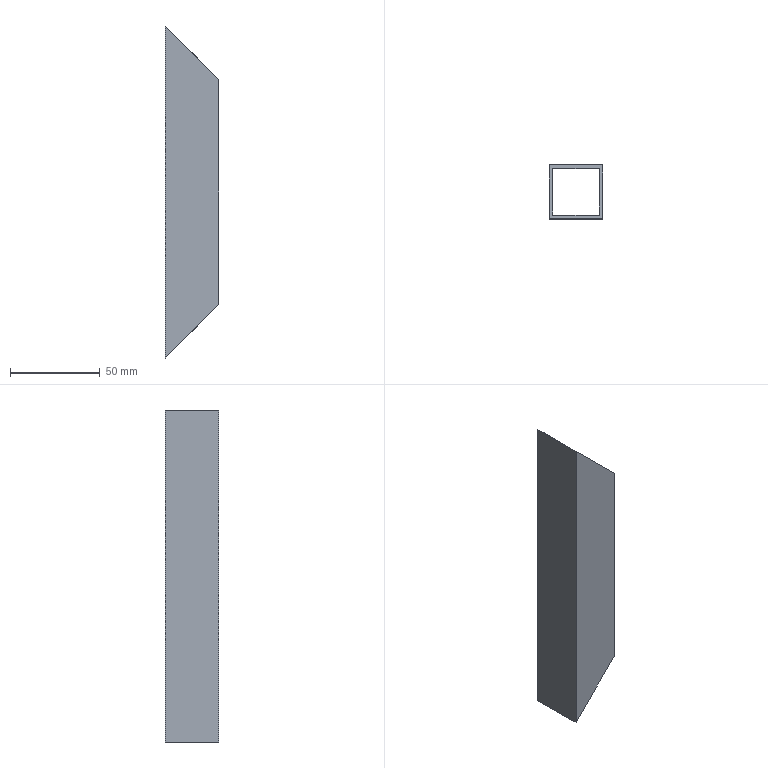Part | SolidWorks | features Extrusion 1, ICE 1 | 1 solid | 10 faces | box 30 x 30 x 185 mm | volume 34720 mm3 | plane 10
STEP:
#1=CARTESIAN_POINT('',(13.,-13.,64.5));
#2=VERTEX_POINT('',#1);
#3=CARTESIAN_POINT('',(-13.,-13.,90.5));
#4=VERTEX_POINT('',#3);
#5=CARTESIAN_POINT('',(-1.,-13.,78.5));
#6=DIRECTION('',(-0.7071,0.,0.7071));
#7=VECTOR('',#6,1000.);
#8=LINE('',#5,#7);
#9=EDGE_CURVE('',#2,#4,#8,.T.);
#10=ORIENTED_EDGE('',*,*,#9,.F.);
#11=CARTESIAN_POINT('',(13.,-13.,-64.5));
#12=VERTEX_POINT('',#11);
#13=CARTESIAN_POINT('',(13.,-13.,92.5));
#14=DIRECTION('',(0.,0.,-1.));
#15=VECTOR('',#14,1000.);
#16=LINE('',#13,#15);
#17=EDGE_CURVE('',#2,#12,#16,.T.);
#18=ORIENTED_EDGE('',*,*,#17,.T.);
#19=CARTESIAN_POINT('',(-13.,-13.,-90.5));
#20=VERTEX_POINT('',#19);
#21=CARTESIAN_POINT('',(91.5,-13.,14.));
#22=DIRECTION('',(0.7071,0.,0.7071));
#23=VECTOR('',#22,1000.);
#24=LINE('',#21,#23);
#25=EDGE_CURVE('',#20,#12,#24,.T.);
#26=ORIENTED_EDGE('',*,*,#25,.F.);
#27=CARTESIAN_POINT('',(-13.,-13.,92.5));
#28=DIRECTION('',(0.,0.,-1.));
#29=VECTOR('',#28,1000.);
#30=LINE('',#27,#29);
#31=EDGE_CURVE('',#4,#20,#30,.T.);
#32=ORIENTED_EDGE('',*,*,#31,.F.);
#33=EDGE_LOOP('',(#10,#18,#26,#32));
#34=FACE_OUTER_BOUND('',#33,.T.);
#35=CARTESIAN_POINT('',(13.,-13.,92.5));
#36=DIRECTION('',(0.,1.,0.));
#37=DIRECTION('',(0.,0.,1.));
#38=AXIS2_PLACEMENT_3D('',#35,#36,#37);
#39=PLANE('',#38);
#40=ADVANCED_FACE('',(#34),#39,.T.);
#41=CARTESIAN_POINT('',(-13.,13.,90.5));
#42=VERTEX_POINT('',#41);
#43=CARTESIAN_POINT('',(-13.,-13.,90.5));
#44=DIRECTION('',(0.,1.,0.));
#45=VECTOR('',#44,1000.);
#46=LINE('',#43,#45);
#47=EDGE_CURVE('',#4,#42,#46,.T.);
#48=ORIENTED_EDGE('',*,*,#47,.F.);
#49=ORIENTED_EDGE('',*,*,#31,.T.);
#50=CARTESIAN_POINT('',(-13.,13.,-90.5));
#51=VERTEX_POINT('',#50);
#52=CARTESIAN_POINT('',(-13.,-13.,-90.5));
#53=DIRECTION('',(0.,-1.,0.));
#54=VECTOR('',#53,1000.);
#55=LINE('',#52,#54);
#56=EDGE_CURVE('',#51,#20,#55,.T.);
#57=ORIENTED_EDGE('',*,*,#56,.F.);
#58=CARTESIAN_POINT('',(-13.,13.,92.5));
#59=DIRECTION('',(0.,0.,-1.));
#60=VECTOR('',#59,1000.);
#61=LINE('',#58,#60);
#62=EDGE_CURVE('',#42,#51,#61,.T.);
#63=ORIENTED_EDGE('',*,*,#62,.F.);
#64=EDGE_LOOP('',(#48,#49,#57,#63));
#65=FACE_OUTER_BOUND('',#64,.T.);
#66=CARTESIAN_POINT('',(-13.,-13.,92.5));
#67=DIRECTION('',(1.,0.,0.));
#68=DIRECTION('',(0.,0.,-1.));
#69=AXIS2_PLACEMENT_3D('',#66,#67,#68);
#70=PLANE('',#69);
#71=ADVANCED_FACE('',(#65),#70,.T.);
#72=CARTESIAN_POINT('',(13.,13.,64.5));
#73=VERTEX_POINT('',#72);
#74=CARTESIAN_POINT('',(-1.,13.,78.5));
#75=DIRECTION('',(0.7071,0.,-0.7071));
#76=VECTOR('',#75,1000.);
#77=LINE('',#74,#76);
#78=EDGE_CURVE('',#42,#73,#77,.T.);
#79=ORIENTED_EDGE('',*,*,#78,.F.);
#80=ORIENTED_EDGE('',*,*,#62,.T.);
#81=CARTESIAN_POINT('',(13.,13.,-64.5));
#82=VERTEX_POINT('',#81);
#83=CARTESIAN_POINT('',(91.5,13.,14.));
#84=DIRECTION('',(-0.7071,0.,-0.7071));
#85=VECTOR('',#84,1000.);
#86=LINE('',#83,#85);
#87=EDGE_CURVE('',#82,#51,#86,.T.);
#88=ORIENTED_EDGE('',*,*,#87,.F.);
#89=CARTESIAN_POINT('',(13.,13.,92.5));
#90=DIRECTION('',(0.,0.,-1.));
#91=VECTOR('',#90,1000.);
#92=LINE('',#89,#91);
#93=EDGE_CURVE('',#73,#82,#92,.T.);
#94=ORIENTED_EDGE('',*,*,#93,.F.);
#95=EDGE_LOOP('',(#79,#80,#88,#94));
#96=FACE_OUTER_BOUND('',#95,.T.);
#97=CARTESIAN_POINT('',(13.,13.,92.5));
#98=DIRECTION('',(0.,-1.,0.));
#99=DIRECTION('',(1.,0.,0.));
#100=AXIS2_PLACEMENT_3D('',#97,#98,#99);
#101=PLANE('',#100);
#102=ADVANCED_FACE('',(#96),#101,.T.);
#103=CARTESIAN_POINT('',(13.,-13.,64.5));
#104=DIRECTION('',(0.,-1.,0.));
#105=VECTOR('',#104,1000.);
#106=LINE('',#103,#105);
#107=EDGE_CURVE('',#73,#2,#106,.T.);
#108=ORIENTED_EDGE('',*,*,#107,.F.);
#109=ORIENTED_EDGE('',*,*,#93,.T.);
#110=CARTESIAN_POINT('',(13.,-13.,-64.5));
#111=DIRECTION('',(0.,1.,0.));
#112=VECTOR('',#111,1000.);
#113=LINE('',#110,#112);
#114=EDGE_CURVE('',#12,#82,#113,.T.);
#115=ORIENTED_EDGE('',*,*,#114,.F.);
#116=ORIENTED_EDGE('',*,*,#17,.F.);
#117=EDGE_LOOP('',(#108,#109,#115,#116));
#118=FACE_OUTER_BOUND('',#117,.T.);
#119=CARTESIAN_POINT('',(13.,-13.,92.5));
#120=DIRECTION('',(-1.,0.,0.));
#121=DIRECTION('',(0.,0.,1.));
#122=AXIS2_PLACEMENT_3D('',#119,#120,#121);
#123=PLANE('',#122);
#124=ADVANCED_FACE('',(#118),#123,.T.);
#125=ORIENTED_EDGE('',*,*,#114,.T.);
#126=ORIENTED_EDGE('',*,*,#87,.T.);
#127=ORIENTED_EDGE('',*,*,#56,.T.);
#128=ORIENTED_EDGE('',*,*,#25,.T.);
#129=EDGE_LOOP('',(#125,#126,#127,#128));
#130=FACE_BOUND('',#129,.T.);
#131=CARTESIAN_POINT('',(-15.,15.,-92.5));
#132=VERTEX_POINT('',#131);
#133=CARTESIAN_POINT('',(-15.,-15.,-92.5));
#134=VERTEX_POINT('',#133);
#135=CARTESIAN_POINT('',(-15.,-15.,-92.5));
#136=DIRECTION('',(0.,-1.,0.));
#137=VECTOR('',#136,1000.);
#138=LINE('',#135,#137);
#139=EDGE_CURVE('',#132,#134,#138,.T.);
#140=ORIENTED_EDGE('',*,*,#139,.F.);
#141=CARTESIAN_POINT('',(15.,15.,-62.5));
#142=VERTEX_POINT('',#141);
#143=CARTESIAN_POINT('',(38.75,15.,-38.75));
#144=DIRECTION('',(0.7071,0.,0.7071));
#145=VECTOR('',#144,1000.);
#146=LINE('',#143,#145);
#147=EDGE_CURVE('',#132,#142,#146,.T.);
#148=ORIENTED_EDGE('',*,*,#147,.T.);
#149=CARTESIAN_POINT('',(15.,-15.,-62.5));
#150=VERTEX_POINT('',#149);
#151=CARTESIAN_POINT('',(15.,-72.,-62.5));
#152=DIRECTION('',(0.,1.,0.));
#153=VECTOR('',#152,1000.);
#154=LINE('',#151,#153);
#155=EDGE_CURVE('',#150,#142,#154,.T.);
#156=ORIENTED_EDGE('',*,*,#155,.F.);
#157=CARTESIAN_POINT('',(92.5,-15.,15.));
#158=DIRECTION('',(0.7071,0.,0.7071));
#159=VECTOR('',#158,1000.);
#160=LINE('',#157,#159);
#161=EDGE_CURVE('',#134,#150,#160,.T.);
#162=ORIENTED_EDGE('',*,*,#161,.F.);
#163=EDGE_LOOP('',(#140,#148,#156,#162));
#164=FACE_OUTER_BOUND('',#163,.T.);
#165=CARTESIAN_POINT('',(38.75,-72.,-38.75));
#166=DIRECTION('',(-0.7071,0.,0.7071));
#167=DIRECTION('',(0.7071,0.,0.7071));
#168=AXIS2_PLACEMENT_3D('',#165,#166,#167);
#169=PLANE('',#168);
#170=ADVANCED_FACE('',(#130,#164),#169,.F.);
#171=ORIENTED_EDGE('',*,*,#107,.T.);
#172=ORIENTED_EDGE('',*,*,#9,.T.);
#173=ORIENTED_EDGE('',*,*,#47,.T.);
#174=ORIENTED_EDGE('',*,*,#78,.T.);
#175=EDGE_LOOP('',(#171,#172,#173,#174));
#176=FACE_BOUND('',#175,.T.);
#177=CARTESIAN_POINT('',(15.,-15.,62.5));
#178=VERTEX_POINT('',#177);
#179=CARTESIAN_POINT('',(15.,15.,62.5));
#180=VERTEX_POINT('',#179);
#181=CARTESIAN_POINT('',(15.,-72.,62.5));
#182=DIRECTION('',(0.,1.,0.));
#183=VECTOR('',#182,1000.);
#184=LINE('',#181,#183);
#185=EDGE_CURVE('',#178,#180,#184,.T.);
#186=ORIENTED_EDGE('',*,*,#185,.T.);
#187=CARTESIAN_POINT('',(-15.,15.,92.5));
#188=VERTEX_POINT('',#187);
#189=CARTESIAN_POINT('',(38.75,15.,38.75));
#190=DIRECTION('',(-0.7071,0.,0.7071));
#191=VECTOR('',#190,1000.);
#192=LINE('',#189,#191);
#193=EDGE_CURVE('',#180,#188,#192,.T.);
#194=ORIENTED_EDGE('',*,*,#193,.T.);
#195=CARTESIAN_POINT('',(-15.,-15.,92.5));
#196=VERTEX_POINT('',#195);
#197=CARTESIAN_POINT('',(-15.,-15.,92.5));
#198=DIRECTION('',(0.,-1.,0.));
#199=VECTOR('',#198,1000.);
#200=LINE('',#197,#199);
#201=EDGE_CURVE('',#188,#196,#200,.T.);
#202=ORIENTED_EDGE('',*,*,#201,.T.);
#203=CARTESIAN_POINT('',(0.,-15.,77.5));
#204=DIRECTION('',(-0.7071,0.,0.7071));
#205=VECTOR('',#204,1000.);
#206=LINE('',#203,#205);
#207=EDGE_CURVE('',#178,#196,#206,.T.);
#208=ORIENTED_EDGE('',*,*,#207,.F.);
#209=EDGE_LOOP('',(#186,#194,#202,#208));
#210=FACE_OUTER_BOUND('',#209,.T.);
#211=CARTESIAN_POINT('',(38.75,-72.,38.75));
#212=DIRECTION('',(-0.7071,0.,-0.7071));
#213=DIRECTION('',(-0.7071,0.,0.7071));
#214=AXIS2_PLACEMENT_3D('',#211,#212,#213);
#215=PLANE('',#214);
#216=ADVANCED_FACE('',(#176,#210),#215,.F.);
#217=ORIENTED_EDGE('',*,*,#139,.T.);
#218=CARTESIAN_POINT('',(-15.,-15.,92.5));
#219=DIRECTION('',(0.,0.,-1.));
#220=VECTOR('',#219,1000.);
#221=LINE('',#218,#220);
#222=EDGE_CURVE('',#196,#134,#221,.T.);
#223=ORIENTED_EDGE('',*,*,#222,.F.);
#224=ORIENTED_EDGE('',*,*,#201,.F.);
#225=CARTESIAN_POINT('',(-15.,15.,92.5));
#226=DIRECTION('',(0.,0.,-1.));
#227=VECTOR('',#226,1000.);
#228=LINE('',#225,#227);
#229=EDGE_CURVE('',#188,#132,#228,.T.);
#230=ORIENTED_EDGE('',*,*,#229,.T.);
#231=EDGE_LOOP('',(#217,#223,#224,#230));
#232=FACE_OUTER_BOUND('',#231,.T.);
#233=CARTESIAN_POINT('',(-15.,-15.,92.5));
#234=DIRECTION('',(1.,0.,0.));
#235=DIRECTION('',(0.,0.,-1.));
#236=AXIS2_PLACEMENT_3D('',#233,#234,#235);
#237=PLANE('',#236);
#238=ADVANCED_FACE('',(#232),#237,.F.);
#239=CARTESIAN_POINT('',(15.,-15.,92.5));
#240=DIRECTION('',(0.,0.,-1.));
#241=VECTOR('',#240,1000.);
#242=LINE('',#239,#241);
#243=EDGE_CURVE('',#178,#150,#242,.T.);
#244=ORIENTED_EDGE('',*,*,#243,.F.);
#245=ORIENTED_EDGE('',*,*,#207,.T.);
#246=ORIENTED_EDGE('',*,*,#222,.T.);
#247=ORIENTED_EDGE('',*,*,#161,.T.);
#248=EDGE_LOOP('',(#244,#245,#246,#247));
#249=FACE_OUTER_BOUND('',#248,.T.);
#250=CARTESIAN_POINT('',(15.,-15.,92.5));
#251=DIRECTION('',(0.,1.,0.));
#252=DIRECTION('',(-1.,0.,0.));
#253=AXIS2_PLACEMENT_3D('',#250,#251,#252);
#254=PLANE('',#253);
#255=ADVANCED_FACE('',(#249),#254,.F.);
#256=CARTESIAN_POINT('',(15.,15.,92.5));
#257=DIRECTION('',(0.,0.,-1.));
#258=VECTOR('',#257,1000.);
#259=LINE('',#256,#258);
#260=EDGE_CURVE('',#180,#142,#259,.T.);
#261=ORIENTED_EDGE('',*,*,#260,.F.);
#262=ORIENTED_EDGE('',*,*,#185,.F.);
#263=ORIENTED_EDGE('',*,*,#243,.T.);
#264=ORIENTED_EDGE('',*,*,#155,.T.);
#265=EDGE_LOOP('',(#261,#262,#263,#264));
#266=FACE_OUTER_BOUND('',#265,.T.);
#267=CARTESIAN_POINT('',(15.,-15.,92.5));
#268=DIRECTION('',(-1.,0.,0.));
#269=DIRECTION('',(0.,0.,1.));
#270=AXIS2_PLACEMENT_3D('',#267,#268,#269);
#271=PLANE('',#270);
#272=ADVANCED_FACE('',(#266),#271,.F.);
#273=ORIENTED_EDGE('',*,*,#229,.F.);
#274=ORIENTED_EDGE('',*,*,#193,.F.);
#275=ORIENTED_EDGE('',*,*,#260,.T.);
#276=ORIENTED_EDGE('',*,*,#147,.F.);
#277=EDGE_LOOP('',(#273,#274,#275,#276));
#278=FACE_OUTER_BOUND('',#277,.T.);
#279=CARTESIAN_POINT('',(15.,15.,92.5));
#280=DIRECTION('',(0.,-1.,0.));
#281=DIRECTION('',(1.,0.,0.));
#282=AXIS2_PLACEMENT_3D('',#279,#280,#281);
#283=PLANE('',#282);
#284=ADVANCED_FACE('',(#278),#283,.F.);
#285=CLOSED_SHELL('',(#40,#71,#102,#124,#170,#216,#238,#255,#272,#284));
#286=MANIFOLD_SOLID_BREP('',#285);
#287=CARTESIAN_POINT('',(0.,0.,0.));
#288=DIRECTION('',(0.,0.,1.));
#289=DIRECTION('',(1.,0.,0.));
#290=AXIS2_PLACEMENT_3D('',#287,#288,#289);
#291=(LENGTH_UNIT()NAMED_UNIT(*)SI_UNIT(.MILLI.,.METRE.));
#292=UNCERTAINTY_MEASURE_WITH_UNIT(LENGTH_MEASURE(0.00001),#291,'','');
#293=(NAMED_UNIT(*)PLANE_ANGLE_UNIT()SI_UNIT($,.RADIAN.));
#294=(NAMED_UNIT(*)SI_UNIT($,.STERADIAN.)SOLID_ANGLE_UNIT());
#295=(GEOMETRIC_REPRESENTATION_CONTEXT(3)GLOBAL_UNCERTAINTY_ASSIGNED_CONTEXT((#292))GLOBAL_UNIT_ASSIGNED_CONTEXT((#291,#293,#294))REPRESENTATION_CONTEXT('',''));
#296=ADVANCED_BREP_SHAPE_REPRESENTATION('',(#286,#290),#295);